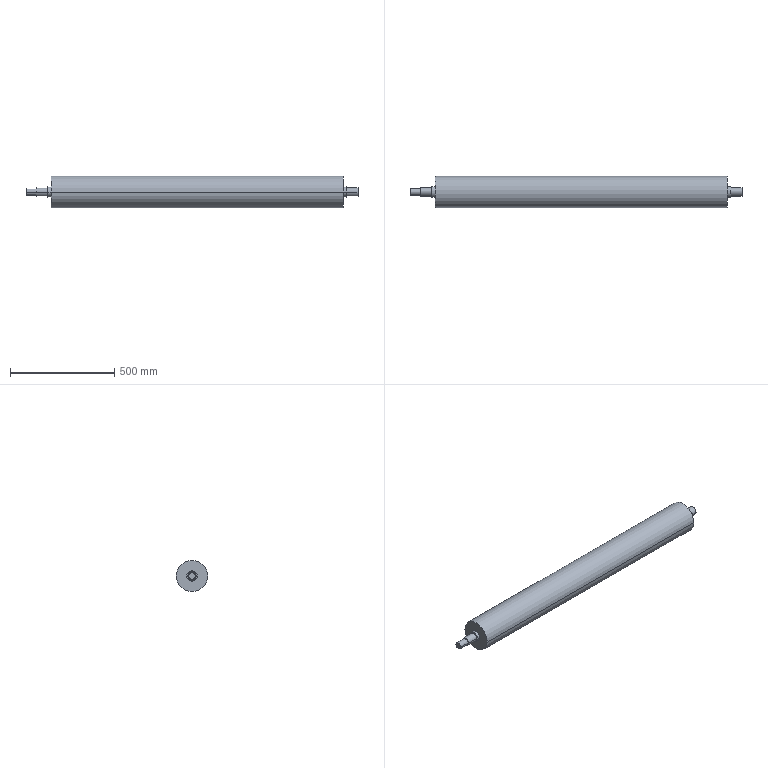Part | SolidWorks | features BaseBody 1 | 1 solid | 19 faces | box 1590 x 150 x 150 mm | volume 24977389 mm3 | cylinder 12 | plane 7 | commonest cylinder face diameters 40 x4 50 x4 32 x2 150 x2
STEP:
#1=CARTESIAN_POINT('',(-770.,-16.,0.));
#2=VERTEX_POINT('',#1);
#3=CARTESIAN_POINT('',(-770.,16.,0.));
#4=VERTEX_POINT('',#3);
#5=CARTESIAN_POINT('',(-770.,0.,0.));
#6=DIRECTION('',(-1.,0.,0.));
#7=DIRECTION('',(0.,-1.,0.));
#8=AXIS2_PLACEMENT_3D('',#5,#6,#7);
#9=CIRCLE('',#8,16.);
#10=EDGE_CURVE('',#2,#4,#9,.T.);
#11=ORIENTED_EDGE('',*,*,#10,.T.);
#12=CARTESIAN_POINT('',(-820.,16.,0.));
#13=VERTEX_POINT('',#12);
#14=CARTESIAN_POINT('',(-810.,16.,0.));
#15=DIRECTION('',(-1.,0.,0.));
#16=VECTOR('',#15,1000.);
#17=LINE('',#14,#16);
#18=EDGE_CURVE('',#4,#13,#17,.T.);
#19=ORIENTED_EDGE('',*,*,#18,.T.);
#20=CARTESIAN_POINT('',(-820.,-16.,0.));
#21=VERTEX_POINT('',#20);
#22=CARTESIAN_POINT('',(-820.,0.,0.));
#23=DIRECTION('',(-1.,0.,0.));
#24=DIRECTION('',(0.,-1.,0.));
#25=AXIS2_PLACEMENT_3D('',#22,#23,#24);
#26=CIRCLE('',#25,16.);
#27=EDGE_CURVE('',#21,#13,#26,.T.);
#28=ORIENTED_EDGE('',*,*,#27,.F.);
#29=CARTESIAN_POINT('',(-810.,-16.,0.));
#30=DIRECTION('',(-1.,0.,0.));
#31=VECTOR('',#30,1000.);
#32=LINE('',#29,#31);
#33=EDGE_CURVE('',#2,#21,#32,.T.);
#34=ORIENTED_EDGE('',*,*,#33,.F.);
#35=EDGE_LOOP('',(#11,#19,#28,#34));
#36=FACE_OUTER_BOUND('',#35,.T.);
#37=CARTESIAN_POINT('',(-810.,0.,0.));
#38=DIRECTION('',(-1.,0.,0.));
#39=DIRECTION('',(0.,-1.,0.));
#40=AXIS2_PLACEMENT_3D('',#37,#38,#39);
#41=CYLINDRICAL_SURFACE('',#40,16.);
#42=ADVANCED_FACE('',(#36),#41,.T.);
#43=CARTESIAN_POINT('',(770.,-20.,0.));
#44=VERTEX_POINT('',#43);
#45=CARTESIAN_POINT('',(770.,20.,0.));
#46=VERTEX_POINT('',#45);
#47=CARTESIAN_POINT('',(770.,0.,0.));
#48=DIRECTION('',(-1.,0.,0.));
#49=DIRECTION('',(0.,-1.,0.));
#50=AXIS2_PLACEMENT_3D('',#47,#48,#49);
#51=CIRCLE('',#50,20.);
#52=EDGE_CURVE('',#44,#46,#51,.T.);
#53=ORIENTED_EDGE('',*,*,#52,.T.);
#54=CARTESIAN_POINT('',(715.,20.,0.));
#55=VERTEX_POINT('',#54);
#56=CARTESIAN_POINT('',(-820.,20.,0.));
#57=DIRECTION('',(-1.,0.,0.));
#58=VECTOR('',#57,1000.);
#59=LINE('',#56,#58);
#60=EDGE_CURVE('',#46,#55,#59,.T.);
#61=ORIENTED_EDGE('',*,*,#60,.T.);
#62=CARTESIAN_POINT('',(715.,-20.,0.));
#63=VERTEX_POINT('',#62);
#64=CARTESIAN_POINT('',(715.,0.,0.));
#65=DIRECTION('',(1.,0.,0.));
#66=DIRECTION('',(0.,-1.,0.));
#67=AXIS2_PLACEMENT_3D('',#64,#65,#66);
#68=CIRCLE('',#67,20.);
#69=EDGE_CURVE('',#55,#63,#68,.T.);
#70=ORIENTED_EDGE('',*,*,#69,.T.);
#71=CARTESIAN_POINT('',(-820.,-20.,0.));
#72=DIRECTION('',(-1.,0.,0.));
#73=VECTOR('',#72,1000.);
#74=LINE('',#71,#73);
#75=EDGE_CURVE('',#44,#63,#74,.T.);
#76=ORIENTED_EDGE('',*,*,#75,.F.);
#77=EDGE_LOOP('',(#53,#61,#70,#76));
#78=FACE_OUTER_BOUND('',#77,.T.);
#79=CARTESIAN_POINT('',(-820.,0.,0.));
#80=DIRECTION('',(-1.,0.,0.));
#81=DIRECTION('',(0.,-1.,0.));
#82=AXIS2_PLACEMENT_3D('',#79,#80,#81);
#83=CYLINDRICAL_SURFACE('',#82,20.);
#84=ADVANCED_FACE('',(#78),#83,.T.);
#85=CARTESIAN_POINT('',(715.,-25.,0.));
#86=VERTEX_POINT('',#85);
#87=CARTESIAN_POINT('',(715.,25.,0.));
#88=VERTEX_POINT('',#87);
#89=CARTESIAN_POINT('',(715.,0.,0.));
#90=DIRECTION('',(-1.,0.,0.));
#91=DIRECTION('',(0.,-1.,0.));
#92=AXIS2_PLACEMENT_3D('',#89,#90,#91);
#93=CIRCLE('',#92,25.);
#94=EDGE_CURVE('',#86,#88,#93,.T.);
#95=ORIENTED_EDGE('',*,*,#94,.T.);
#96=CARTESIAN_POINT('',(700.,25.,0.));
#97=VERTEX_POINT('',#96);
#98=CARTESIAN_POINT('',(-820.,25.,0.));
#99=DIRECTION('',(-1.,0.,0.));
#100=VECTOR('',#99,1000.);
#101=LINE('',#98,#100);
#102=EDGE_CURVE('',#88,#97,#101,.T.);
#103=ORIENTED_EDGE('',*,*,#102,.T.);
#104=CARTESIAN_POINT('',(700.,-25.,0.));
#105=VERTEX_POINT('',#104);
#106=CARTESIAN_POINT('',(700.,0.,0.));
#107=DIRECTION('',(1.,0.,0.));
#108=DIRECTION('',(0.,-1.,0.));
#109=AXIS2_PLACEMENT_3D('',#106,#107,#108);
#110=CIRCLE('',#109,25.);
#111=EDGE_CURVE('',#97,#105,#110,.T.);
#112=ORIENTED_EDGE('',*,*,#111,.T.);
#113=CARTESIAN_POINT('',(-820.,-25.,0.));
#114=DIRECTION('',(-1.,0.,0.));
#115=VECTOR('',#114,1000.);
#116=LINE('',#113,#115);
#117=EDGE_CURVE('',#86,#105,#116,.T.);
#118=ORIENTED_EDGE('',*,*,#117,.F.);
#119=EDGE_LOOP('',(#95,#103,#112,#118));
#120=FACE_OUTER_BOUND('',#119,.T.);
#121=CARTESIAN_POINT('',(-820.,0.,0.));
#122=DIRECTION('',(-1.,0.,0.));
#123=DIRECTION('',(0.,-1.,0.));
#124=AXIS2_PLACEMENT_3D('',#121,#122,#123);
#125=CYLINDRICAL_SURFACE('',#124,25.);
#126=ADVANCED_FACE('',(#120),#125,.T.);
#127=CARTESIAN_POINT('',(-700.,-25.,0.));
#128=VERTEX_POINT('',#127);
#129=CARTESIAN_POINT('',(-700.,25.,0.));
#130=VERTEX_POINT('',#129);
#131=CARTESIAN_POINT('',(-700.,0.,0.));
#132=DIRECTION('',(-1.,0.,0.));
#133=DIRECTION('',(0.,1.,0.));
#134=AXIS2_PLACEMENT_3D('',#131,#132,#133);
#135=CIRCLE('',#134,25.);
#136=EDGE_CURVE('',#128,#130,#135,.T.);
#137=ORIENTED_EDGE('',*,*,#136,.T.);
#138=CARTESIAN_POINT('',(-715.,25.,0.));
#139=VERTEX_POINT('',#138);
#140=CARTESIAN_POINT('',(-820.,25.,0.));
#141=DIRECTION('',(-1.,0.,0.));
#142=VECTOR('',#141,1000.);
#143=LINE('',#140,#142);
#144=EDGE_CURVE('',#130,#139,#143,.T.);
#145=ORIENTED_EDGE('',*,*,#144,.T.);
#146=CARTESIAN_POINT('',(-715.,-25.,0.));
#147=VERTEX_POINT('',#146);
#148=CARTESIAN_POINT('',(-715.,0.,0.));
#149=DIRECTION('',(-1.,0.,0.));
#150=DIRECTION('',(0.,-1.,0.));
#151=AXIS2_PLACEMENT_3D('',#148,#149,#150);
#152=CIRCLE('',#151,25.);
#153=EDGE_CURVE('',#147,#139,#152,.T.);
#154=ORIENTED_EDGE('',*,*,#153,.F.);
#155=CARTESIAN_POINT('',(-820.,-25.,0.));
#156=DIRECTION('',(-1.,0.,0.));
#157=VECTOR('',#156,1000.);
#158=LINE('',#155,#157);
#159=EDGE_CURVE('',#128,#147,#158,.T.);
#160=ORIENTED_EDGE('',*,*,#159,.F.);
#161=EDGE_LOOP('',(#137,#145,#154,#160));
#162=FACE_OUTER_BOUND('',#161,.T.);
#163=CARTESIAN_POINT('',(-820.,0.,0.));
#164=DIRECTION('',(-1.,0.,0.));
#165=DIRECTION('',(0.,-1.,0.));
#166=AXIS2_PLACEMENT_3D('',#163,#164,#165);
#167=CYLINDRICAL_SURFACE('',#166,25.);
#168=ADVANCED_FACE('',(#162),#167,.T.);
#169=CARTESIAN_POINT('',(700.,-75.,0.));
#170=VERTEX_POINT('',#169);
#171=CARTESIAN_POINT('',(700.,75.,0.));
#172=VERTEX_POINT('',#171);
#173=CARTESIAN_POINT('',(700.,0.,0.));
#174=DIRECTION('',(-1.,0.,0.));
#175=DIRECTION('',(0.,-1.,0.));
#176=AXIS2_PLACEMENT_3D('',#173,#174,#175);
#177=CIRCLE('',#176,75.);
#178=EDGE_CURVE('',#170,#172,#177,.T.);
#179=ORIENTED_EDGE('',*,*,#178,.T.);
#180=CARTESIAN_POINT('',(-700.,75.,0.));
#181=VERTEX_POINT('',#180);
#182=CARTESIAN_POINT('',(-820.,75.,0.));
#183=DIRECTION('',(-1.,0.,0.));
#184=VECTOR('',#183,1000.);
#185=LINE('',#182,#184);
#186=EDGE_CURVE('',#172,#181,#185,.T.);
#187=ORIENTED_EDGE('',*,*,#186,.T.);
#188=CARTESIAN_POINT('',(-700.,-75.,0.));
#189=VERTEX_POINT('',#188);
#190=CARTESIAN_POINT('',(-700.,0.,0.));
#191=DIRECTION('',(-1.,0.,0.));
#192=DIRECTION('',(0.,-1.,0.));
#193=AXIS2_PLACEMENT_3D('',#190,#191,#192);
#194=CIRCLE('',#193,75.);
#195=EDGE_CURVE('',#189,#181,#194,.T.);
#196=ORIENTED_EDGE('',*,*,#195,.F.);
#197=CARTESIAN_POINT('',(-820.,-75.,0.));
#198=DIRECTION('',(-1.,0.,0.));
#199=VECTOR('',#198,1000.);
#200=LINE('',#197,#199);
#201=EDGE_CURVE('',#170,#189,#200,.T.);
#202=ORIENTED_EDGE('',*,*,#201,.F.);
#203=EDGE_LOOP('',(#179,#187,#196,#202));
#204=FACE_OUTER_BOUND('',#203,.T.);
#205=CARTESIAN_POINT('',(-820.,0.,0.));
#206=DIRECTION('',(-1.,0.,0.));
#207=DIRECTION('',(0.,-1.,0.));
#208=AXIS2_PLACEMENT_3D('',#205,#206,#207);
#209=CYLINDRICAL_SURFACE('',#208,75.);
#210=ADVANCED_FACE('',(#204),#209,.T.);
#211=CARTESIAN_POINT('',(-715.,-20.,0.));
#212=VERTEX_POINT('',#211);
#213=CARTESIAN_POINT('',(-715.,20.,0.));
#214=VERTEX_POINT('',#213);
#215=CARTESIAN_POINT('',(-715.,0.,0.));
#216=DIRECTION('',(-1.,0.,0.));
#217=DIRECTION('',(0.,1.,0.));
#218=AXIS2_PLACEMENT_3D('',#215,#216,#217);
#219=CIRCLE('',#218,20.);
#220=EDGE_CURVE('',#212,#214,#219,.T.);
#221=ORIENTED_EDGE('',*,*,#220,.T.);
#222=CARTESIAN_POINT('',(-770.,20.,0.));
#223=VERTEX_POINT('',#222);
#224=CARTESIAN_POINT('',(-820.,20.,0.));
#225=DIRECTION('',(-1.,0.,0.));
#226=VECTOR('',#225,1000.);
#227=LINE('',#224,#226);
#228=EDGE_CURVE('',#214,#223,#227,.T.);
#229=ORIENTED_EDGE('',*,*,#228,.T.);
#230=CARTESIAN_POINT('',(-770.,-20.,0.));
#231=VERTEX_POINT('',#230);
#232=CARTESIAN_POINT('',(-770.,0.,0.));
#233=DIRECTION('',(-1.,0.,0.));
#234=DIRECTION('',(0.,-1.,0.));
#235=AXIS2_PLACEMENT_3D('',#232,#233,#234);
#236=CIRCLE('',#235,20.);
#237=EDGE_CURVE('',#231,#223,#236,.T.);
#238=ORIENTED_EDGE('',*,*,#237,.F.);
#239=CARTESIAN_POINT('',(-820.,-20.,0.));
#240=DIRECTION('',(-1.,0.,0.));
#241=VECTOR('',#240,1000.);
#242=LINE('',#239,#241);
#243=EDGE_CURVE('',#212,#231,#242,.T.);
#244=ORIENTED_EDGE('',*,*,#243,.F.);
#245=EDGE_LOOP('',(#221,#229,#238,#244));
#246=FACE_OUTER_BOUND('',#245,.T.);
#247=CARTESIAN_POINT('',(-820.,0.,0.));
#248=DIRECTION('',(-1.,0.,0.));
#249=DIRECTION('',(0.,-1.,0.));
#250=AXIS2_PLACEMENT_3D('',#247,#248,#249);
#251=CYLINDRICAL_SURFACE('',#250,20.);
#252=ADVANCED_FACE('',(#246),#251,.T.);
#253=ORIENTED_EDGE('',*,*,#27,.T.);
#254=CARTESIAN_POINT('',(-820.,0.,0.));
#255=DIRECTION('',(-1.,0.,0.));
#256=DIRECTION('',(0.,-1.,0.));
#257=AXIS2_PLACEMENT_3D('',#254,#255,#256);
#258=CIRCLE('',#257,16.);
#259=EDGE_CURVE('',#13,#21,#258,.T.);
#260=ORIENTED_EDGE('',*,*,#259,.T.);
#261=EDGE_LOOP('',(#253,#260));
#262=FACE_OUTER_BOUND('',#261,.T.);
#263=CARTESIAN_POINT('',(-820.,17.5,0.));
#264=DIRECTION('',(1.,0.,0.));
#265=DIRECTION('',(0.,-1.,0.));
#266=AXIS2_PLACEMENT_3D('',#263,#264,#265);
#267=PLANE('',#266);
#268=ADVANCED_FACE('',(#262),#267,.F.);
#269=ORIENTED_EDGE('',*,*,#10,.F.);
#270=CARTESIAN_POINT('',(-770.,0.,0.));
#271=DIRECTION('',(-1.,0.,0.));
#272=DIRECTION('',(0.,-1.,0.));
#273=AXIS2_PLACEMENT_3D('',#270,#271,#272);
#274=CIRCLE('',#273,16.);
#275=EDGE_CURVE('',#4,#2,#274,.T.);
#276=ORIENTED_EDGE('',*,*,#275,.F.);
#277=EDGE_LOOP('',(#269,#276));
#278=FACE_BOUND('',#277,.T.);
#279=ORIENTED_EDGE('',*,*,#237,.T.);
#280=CARTESIAN_POINT('',(-770.,0.,0.));
#281=DIRECTION('',(-1.,0.,0.));
#282=DIRECTION('',(0.,-1.,0.));
#283=AXIS2_PLACEMENT_3D('',#280,#281,#282);
#284=CIRCLE('',#283,20.);
#285=EDGE_CURVE('',#223,#231,#284,.T.);
#286=ORIENTED_EDGE('',*,*,#285,.T.);
#287=EDGE_LOOP('',(#279,#286));
#288=FACE_OUTER_BOUND('',#287,.T.);
#289=CARTESIAN_POINT('',(-770.,0.,0.));
#290=DIRECTION('',(-1.,0.,0.));
#291=DIRECTION('',(0.,0.,1.));
#292=AXIS2_PLACEMENT_3D('',#289,#290,#291);
#293=PLANE('',#292);
#294=ADVANCED_FACE('',(#278,#288),#293,.T.);
#295=ORIENTED_EDGE('',*,*,#52,.F.);
#296=CARTESIAN_POINT('',(770.,0.,0.));
#297=DIRECTION('',(-1.,0.,0.));
#298=DIRECTION('',(0.,-1.,0.));
#299=AXIS2_PLACEMENT_3D('',#296,#297,#298);
#300=CIRCLE('',#299,20.);
#301=EDGE_CURVE('',#46,#44,#300,.T.);
#302=ORIENTED_EDGE('',*,*,#301,.F.);
#303=EDGE_LOOP('',(#295,#302));
#304=FACE_OUTER_BOUND('',#303,.T.);
#305=CARTESIAN_POINT('',(770.,17.5,0.));
#306=DIRECTION('',(-1.,0.,0.));
#307=DIRECTION('',(0.,0.,1.));
#308=AXIS2_PLACEMENT_3D('',#305,#306,#307);
#309=PLANE('',#308);
#310=ADVANCED_FACE('',(#304),#309,.F.);
#311=CARTESIAN_POINT('',(715.,0.,0.));
#312=DIRECTION('',(1.,0.,0.));
#313=DIRECTION('',(0.,-1.,0.));
#314=AXIS2_PLACEMENT_3D('',#311,#312,#313);
#315=CIRCLE('',#314,20.);
#316=EDGE_CURVE('',#63,#55,#315,.T.);
#317=ORIENTED_EDGE('',*,*,#316,.F.);
#318=ORIENTED_EDGE('',*,*,#69,.F.);
#319=EDGE_LOOP('',(#317,#318));
#320=FACE_BOUND('',#319,.T.);
#321=ORIENTED_EDGE('',*,*,#94,.F.);
#322=CARTESIAN_POINT('',(715.,0.,0.));
#323=DIRECTION('',(-1.,0.,0.));
#324=DIRECTION('',(0.,-1.,0.));
#325=AXIS2_PLACEMENT_3D('',#322,#323,#324);
#326=CIRCLE('',#325,25.);
#327=EDGE_CURVE('',#88,#86,#326,.T.);
#328=ORIENTED_EDGE('',*,*,#327,.F.);
#329=EDGE_LOOP('',(#321,#328));
#330=FACE_OUTER_BOUND('',#329,.T.);
#331=CARTESIAN_POINT('',(715.,20.,0.));
#332=DIRECTION('',(-1.,0.,0.));
#333=DIRECTION('',(0.,0.,1.));
#334=AXIS2_PLACEMENT_3D('',#331,#332,#333);
#335=PLANE('',#334);
#336=ADVANCED_FACE('',(#320,#330),#335,.F.);
#337=ORIENTED_EDGE('',*,*,#220,.F.);
#338=CARTESIAN_POINT('',(-715.,0.,0.));
#339=DIRECTION('',(-1.,0.,0.));
#340=DIRECTION('',(0.,1.,0.));
#341=AXIS2_PLACEMENT_3D('',#338,#339,#340);
#342=CIRCLE('',#341,20.);
#343=EDGE_CURVE('',#214,#212,#342,.T.);
#344=ORIENTED_EDGE('',*,*,#343,.F.);
#345=EDGE_LOOP('',(#337,#344));
#346=FACE_BOUND('',#345,.T.);
#347=ORIENTED_EDGE('',*,*,#153,.T.);
#348=CARTESIAN_POINT('',(-715.,0.,0.));
#349=DIRECTION('',(-1.,0.,0.));
#350=DIRECTION('',(0.,-1.,0.));
#351=AXIS2_PLACEMENT_3D('',#348,#349,#350);
#352=CIRCLE('',#351,25.);
#353=EDGE_CURVE('',#139,#147,#352,.T.);
#354=ORIENTED_EDGE('',*,*,#353,.T.);
#355=EDGE_LOOP('',(#347,#354));
#356=FACE_OUTER_BOUND('',#355,.T.);
#357=CARTESIAN_POINT('',(-715.,0.,0.));
#358=DIRECTION('',(1.,0.,0.));
#359=DIRECTION('',(0.,-1.,0.));
#360=AXIS2_PLACEMENT_3D('',#357,#358,#359);
#361=PLANE('',#360);
#362=ADVANCED_FACE('',(#346,#356),#361,.F.);
#363=CARTESIAN_POINT('',(700.,0.,0.));
#364=DIRECTION('',(1.,0.,0.));
#365=DIRECTION('',(0.,-1.,0.));
#366=AXIS2_PLACEMENT_3D('',#363,#364,#365);
#367=CIRCLE('',#366,25.);
#368=EDGE_CURVE('',#105,#97,#367,.T.);
#369=ORIENTED_EDGE('',*,*,#368,.F.);
#370=ORIENTED_EDGE('',*,*,#111,.F.);
#371=EDGE_LOOP('',(#369,#370));
#372=FACE_BOUND('',#371,.T.);
#373=ORIENTED_EDGE('',*,*,#178,.F.);
#374=CARTESIAN_POINT('',(700.,0.,0.));
#375=DIRECTION('',(-1.,0.,0.));
#376=DIRECTION('',(0.,-1.,0.));
#377=AXIS2_PLACEMENT_3D('',#374,#375,#376);
#378=CIRCLE('',#377,75.);
#379=EDGE_CURVE('',#172,#170,#378,.T.);
#380=ORIENTED_EDGE('',*,*,#379,.F.);
#381=EDGE_LOOP('',(#373,#380));
#382=FACE_OUTER_BOUND('',#381,.T.);
#383=CARTESIAN_POINT('',(700.,75.,0.));
#384=DIRECTION('',(-1.,0.,0.));
#385=DIRECTION('',(0.,0.,1.));
#386=AXIS2_PLACEMENT_3D('',#383,#384,#385);
#387=PLANE('',#386);
#388=ADVANCED_FACE('',(#372,#382),#387,.F.);
#389=ORIENTED_EDGE('',*,*,#136,.F.);
#390=CARTESIAN_POINT('',(-700.,0.,0.));
#391=DIRECTION('',(-1.,0.,0.));
#392=DIRECTION('',(0.,1.,0.));
#393=AXIS2_PLACEMENT_3D('',#390,#391,#392);
#394=CIRCLE('',#393,25.);
#395=EDGE_CURVE('',#130,#128,#394,.T.);
#396=ORIENTED_EDGE('',*,*,#395,.F.);
#397=EDGE_LOOP('',(#389,#396));
#398=FACE_BOUND('',#397,.T.);
#399=ORIENTED_EDGE('',*,*,#195,.T.);
#400=CARTESIAN_POINT('',(-700.,0.,0.));
#401=DIRECTION('',(-1.,0.,0.));
#402=DIRECTION('',(0.,-1.,0.));
#403=AXIS2_PLACEMENT_3D('',#400,#401,#402);
#404=CIRCLE('',#403,75.);
#405=EDGE_CURVE('',#181,#189,#404,.T.);
#406=ORIENTED_EDGE('',*,*,#405,.T.);
#407=EDGE_LOOP('',(#399,#406));
#408=FACE_OUTER_BOUND('',#407,.T.);
#409=CARTESIAN_POINT('',(-700.,75.,0.));
#410=DIRECTION('',(1.,0.,0.));
#411=DIRECTION('',(0.,-1.,0.));
#412=AXIS2_PLACEMENT_3D('',#409,#410,#411);
#413=PLANE('',#412);
#414=ADVANCED_FACE('',(#398,#408),#413,.F.);
#415=ORIENTED_EDGE('',*,*,#228,.F.);
#416=ORIENTED_EDGE('',*,*,#343,.T.);
#417=ORIENTED_EDGE('',*,*,#243,.T.);
#418=ORIENTED_EDGE('',*,*,#285,.F.);
#419=EDGE_LOOP('',(#415,#416,#417,#418));
#420=FACE_OUTER_BOUND('',#419,.T.);
#421=CARTESIAN_POINT('',(-820.,0.,0.));
#422=DIRECTION('',(-1.,0.,0.));
#423=DIRECTION('',(0.,-1.,0.));
#424=AXIS2_PLACEMENT_3D('',#421,#422,#423);
#425=CYLINDRICAL_SURFACE('',#424,20.);
#426=ADVANCED_FACE('',(#420),#425,.T.);
#427=ORIENTED_EDGE('',*,*,#186,.F.);
#428=ORIENTED_EDGE('',*,*,#379,.T.);
#429=ORIENTED_EDGE('',*,*,#201,.T.);
#430=ORIENTED_EDGE('',*,*,#405,.F.);
#431=EDGE_LOOP('',(#427,#428,#429,#430));
#432=FACE_OUTER_BOUND('',#431,.T.);
#433=CARTESIAN_POINT('',(-820.,0.,0.));
#434=DIRECTION('',(-1.,0.,0.));
#435=DIRECTION('',(0.,-1.,0.));
#436=AXIS2_PLACEMENT_3D('',#433,#434,#435);
#437=CYLINDRICAL_SURFACE('',#436,75.);
#438=ADVANCED_FACE('',(#432),#437,.T.);
#439=ORIENTED_EDGE('',*,*,#144,.F.);
#440=ORIENTED_EDGE('',*,*,#395,.T.);
#441=ORIENTED_EDGE('',*,*,#159,.T.);
#442=ORIENTED_EDGE('',*,*,#353,.F.);
#443=EDGE_LOOP('',(#439,#440,#441,#442));
#444=FACE_OUTER_BOUND('',#443,.T.);
#445=CARTESIAN_POINT('',(-820.,0.,0.));
#446=DIRECTION('',(-1.,0.,0.));
#447=DIRECTION('',(0.,-1.,0.));
#448=AXIS2_PLACEMENT_3D('',#445,#446,#447);
#449=CYLINDRICAL_SURFACE('',#448,25.);
#450=ADVANCED_FACE('',(#444),#449,.T.);
#451=ORIENTED_EDGE('',*,*,#102,.F.);
#452=ORIENTED_EDGE('',*,*,#327,.T.);
#453=ORIENTED_EDGE('',*,*,#117,.T.);
#454=ORIENTED_EDGE('',*,*,#368,.T.);
#455=EDGE_LOOP('',(#451,#452,#453,#454));
#456=FACE_OUTER_BOUND('',#455,.T.);
#457=CARTESIAN_POINT('',(-820.,0.,0.));
#458=DIRECTION('',(-1.,0.,0.));
#459=DIRECTION('',(0.,-1.,0.));
#460=AXIS2_PLACEMENT_3D('',#457,#458,#459);
#461=CYLINDRICAL_SURFACE('',#460,25.);
#462=ADVANCED_FACE('',(#456),#461,.T.);
#463=ORIENTED_EDGE('',*,*,#60,.F.);
#464=ORIENTED_EDGE('',*,*,#301,.T.);
#465=ORIENTED_EDGE('',*,*,#75,.T.);
#466=ORIENTED_EDGE('',*,*,#316,.T.);
#467=EDGE_LOOP('',(#463,#464,#465,#466));
#468=FACE_OUTER_BOUND('',#467,.T.);
#469=CARTESIAN_POINT('',(-820.,0.,0.));
#470=DIRECTION('',(-1.,0.,0.));
#471=DIRECTION('',(0.,-1.,0.));
#472=AXIS2_PLACEMENT_3D('',#469,#470,#471);
#473=CYLINDRICAL_SURFACE('',#472,20.);
#474=ADVANCED_FACE('',(#468),#473,.T.);
#475=ORIENTED_EDGE('',*,*,#18,.F.);
#476=ORIENTED_EDGE('',*,*,#275,.T.);
#477=ORIENTED_EDGE('',*,*,#33,.T.);
#478=ORIENTED_EDGE('',*,*,#259,.F.);
#479=EDGE_LOOP('',(#475,#476,#477,#478));
#480=FACE_OUTER_BOUND('',#479,.T.);
#481=CARTESIAN_POINT('',(-810.,0.,0.));
#482=DIRECTION('',(-1.,0.,0.));
#483=DIRECTION('',(0.,-1.,0.));
#484=AXIS2_PLACEMENT_3D('',#481,#482,#483);
#485=CYLINDRICAL_SURFACE('',#484,16.);
#486=ADVANCED_FACE('',(#480),#485,.T.);
#487=CLOSED_SHELL('',(#42,#84,#126,#168,#210,#252,#268,#294,#310,#336,#362,#388,#414,#426,#438,#450,#462,#474,#486));
#488=MANIFOLD_SOLID_BREP('',#487);
#489=CARTESIAN_POINT('',(0.,0.,0.));
#490=DIRECTION('',(0.,0.,1.));
#491=DIRECTION('',(1.,0.,0.));
#492=AXIS2_PLACEMENT_3D('',#489,#490,#491);
#493=(LENGTH_UNIT()NAMED_UNIT(*)SI_UNIT(.MILLI.,.METRE.));
#494=UNCERTAINTY_MEASURE_WITH_UNIT(LENGTH_MEASURE(0.00001),#493,'','');
#495=(NAMED_UNIT(*)PLANE_ANGLE_UNIT()SI_UNIT($,.RADIAN.));
#496=(NAMED_UNIT(*)SI_UNIT($,.STERADIAN.)SOLID_ANGLE_UNIT());
#497=(GEOMETRIC_REPRESENTATION_CONTEXT(3)GLOBAL_UNCERTAINTY_ASSIGNED_CONTEXT((#494))GLOBAL_UNIT_ASSIGNED_CONTEXT((#493,#495,#496))REPRESENTATION_CONTEXT('',''));
#498=ADVANCED_BREP_SHAPE_REPRESENTATION('',(#488,#492),#497);